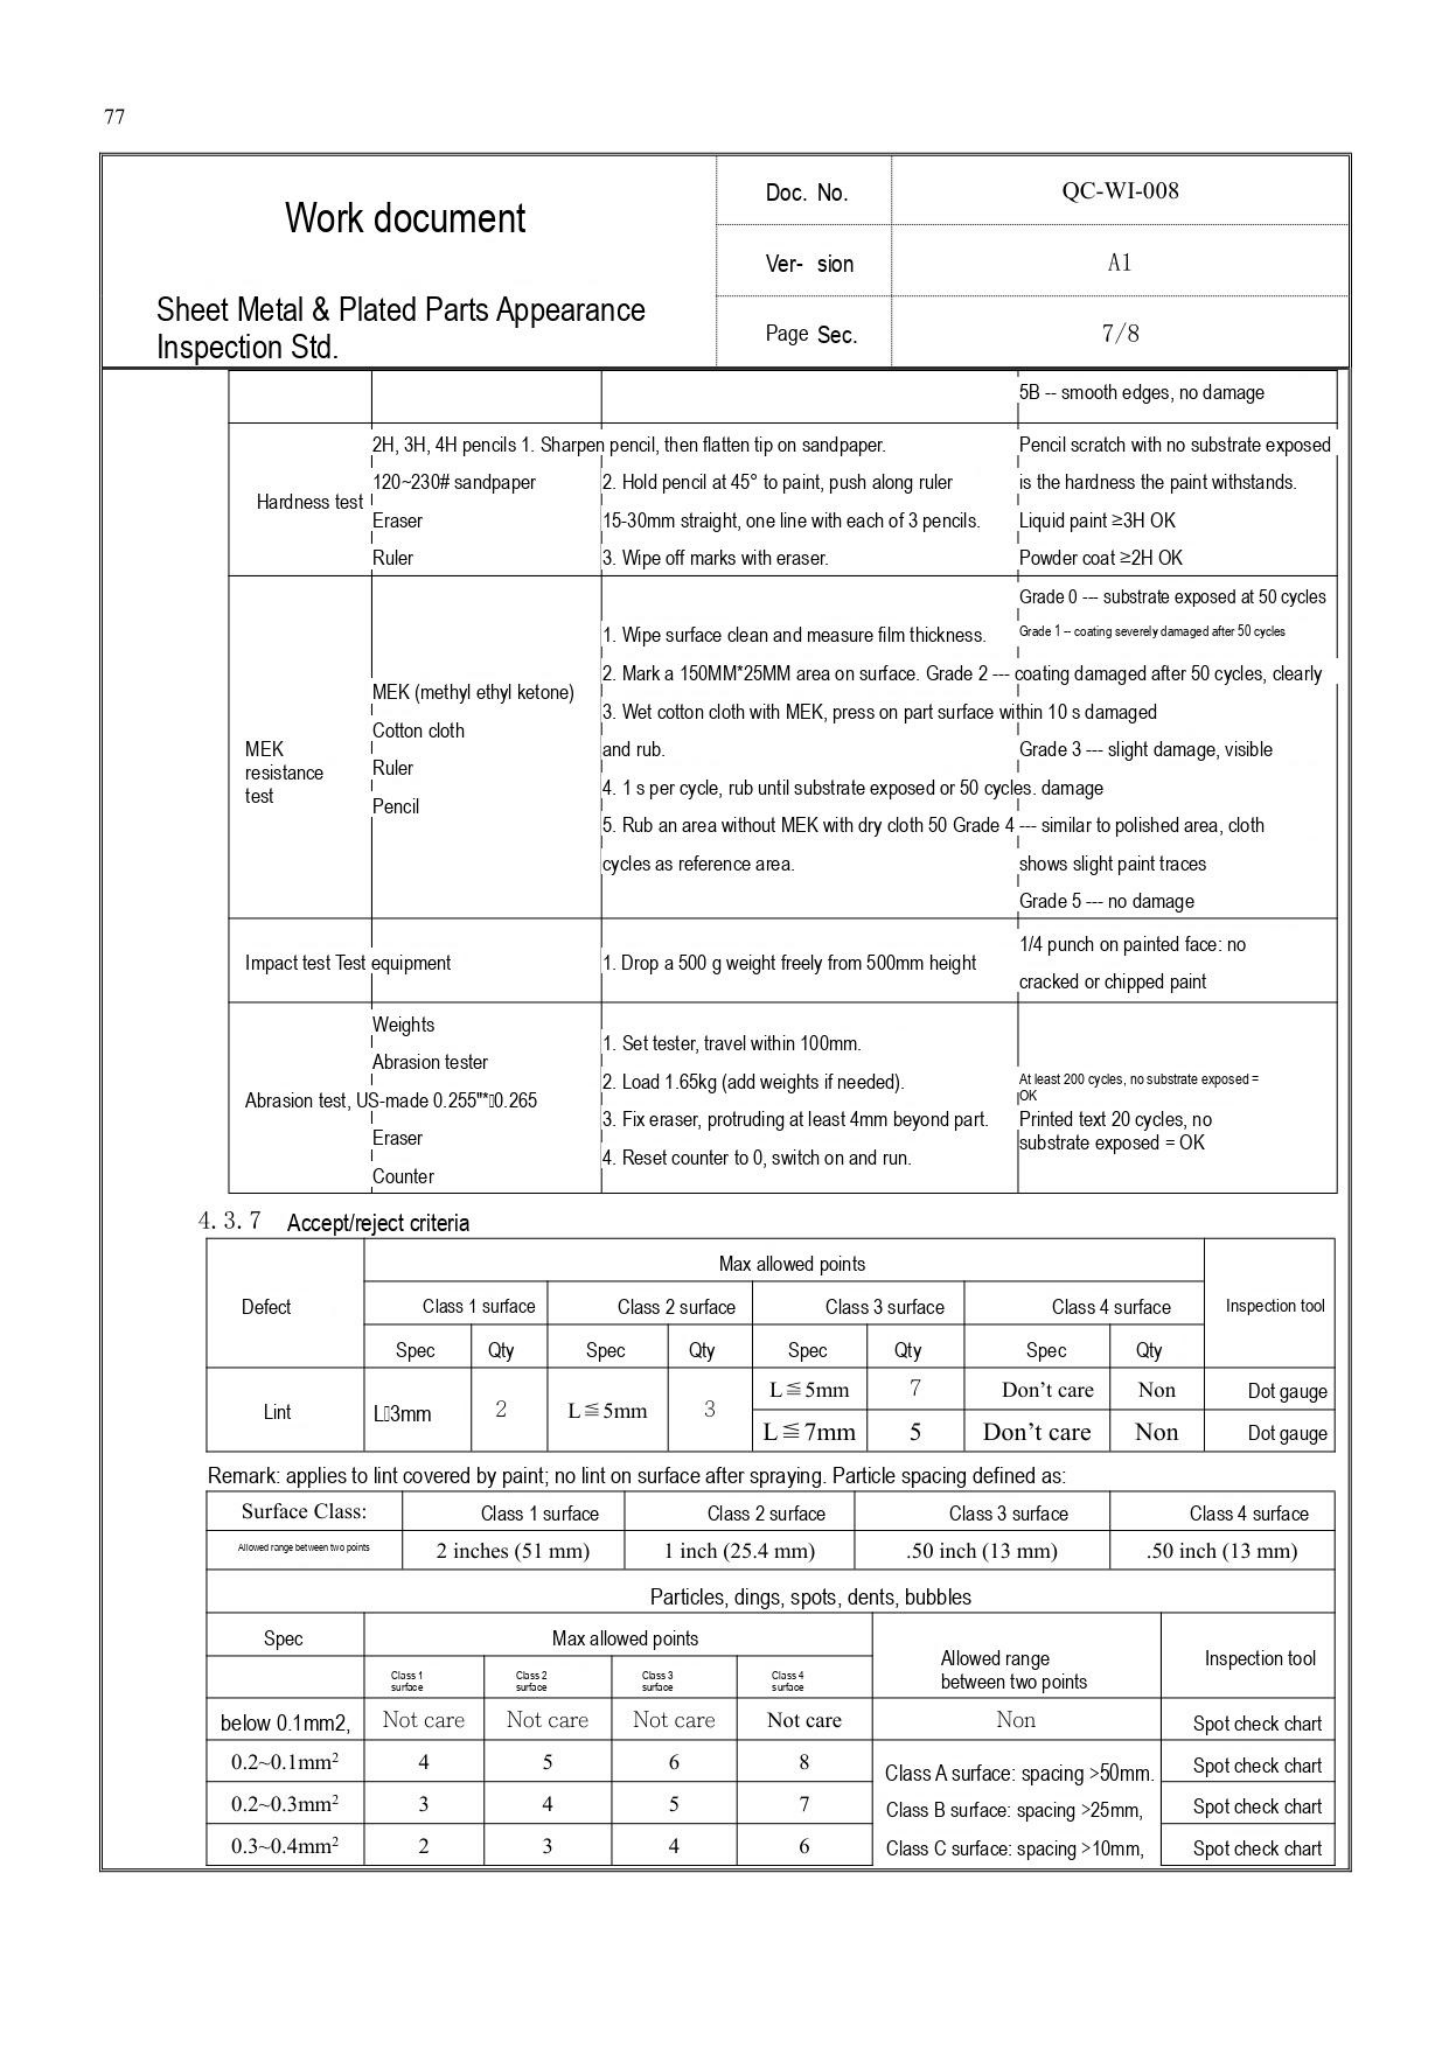77

| Work document<br>Sheet Metal & Plated Parts Appearance Inspection Std. | Doc. No. | QC-WI-008 |
|---|---|---|
| | Ver- sion | A1 |
| | Page Sec. | 7/8 |

| | | | |
|---|---|---|---|
| | | | 5B -- smooth edges, no damage |
| Hardness test | 2H, 3H, 4H pencils<br>120~230# sandpaper<br>Eraser<br>Ruler | 1. Sharpen pencil, then flatten tip on sandpaper.<br>2. Hold pencil at 45° to paint, push along ruler 15-30mm straight, one line with each of 3 pencils.<br>3. Wipe off marks with eraser. | Pencil scratch with no substrate exposed is the hardness the paint withstands.<br>Liquid paint ≥3H OK<br>Powder coat ≥2H OK |
| MEK resistance test | MEK (methyl ethyl ketone)<br>Cotton cloth<br>Ruler<br>Pencil | 1. Wipe surface clean and measure film thickness.<br>2. Mark a 150MM*25MM area on surface.<br>3. Wet cotton cloth with MEK, press on part surface within 10 s and rub.<br>4. 1 s per cycle, rub until substrate exposed or 50 cycles.<br>5. Rub an area without MEK with dry cloth 50 cycles as reference area. | Grade 0 --- substrate exposed at 50 cycles<br>Grade 1 -- coating severely damaged after 50 cycles<br>Grade 2 --- coating damaged after 50 cycles, clearly damaged<br>Grade 3 --- slight damage, visible damage<br>Grade 4 --- similar to polished area, cloth shows slight paint traces<br>Grade 5 --- no damage |
| Impact test | Test equipment | 1. Drop a 500 g weight freely from 500mm height | 1/4 punch on painted face: no cracked or chipped paint |
| Abrasion test, | Weights<br>Abrasion tester<br>US-made 0.255"*0.265<br>Eraser<br>Counter | 1. Set tester, travel within 100mm.<br>2. Load 1.65kg (add weights if needed).<br>3. Fix eraser, protruding at least 4mm beyond part.<br>4. Reset counter to 0, switch on and run. | At least 200 cycles, no substrate exposed = OK<br>Printed text 20 cycles, no substrate exposed = OK |

4.3.7 Accept/reject criteria

| Defect | Max allowed points | | | | | | | | Inspection tool |
|---|---|---|---|---|---|---|---|---|---|
| | Class 1 surface | | Class 2 surface | | Class 3 surface | | Class 4 surface | | |
| | Spec | Qty | Spec | Qty | Spec | Qty | Spec | Qty | |
| Lint | L3mm | 2 | L≦5mm | 3 | L≦5mm | 7 | Don't care | Non | Dot gauge |
| | | | | | L≦7mm | 5 | Don't care | Non | Dot gauge |

Remark: applies to lint covered by paint; no lint on surface after spraying. Particle spacing defined as:

| Surface Class: | Class 1 surface | Class 2 surface | Class 3 surface | Class 4 surface |
|---|---|---|---|---|
| Allowed range between two points | 2 inches (51 mm) | 1 inch (25.4 mm) | .50 inch (13 mm) | .50 inch (13 mm) |

Particles, dings, spots, dents, bubbles

| Spec | Max allowed points | | | | Allowed range between two points | Inspection tool |
|---|---|---|---|---|---|---|
| | Class 1 surface | Class 2 surface | Class 3 surface | Class 4 surface | | |
| below 0.1mm2, | Not care | Not care | Not care | Not care | Non | Spot check chart |
| 0.2~0.1mm² | 4 | 5 | 6 | 8 | Class A surface: spacing >50mm. | Spot check chart |
| 0.2~0.3mm² | 3 | 4 | 5 | 7 | Class B surface: spacing >25mm, | Spot check chart |
| 0.3~0.4mm² | 2 | 3 | 4 | 6 | Class C surface: spacing >10mm, | Spot check chart |
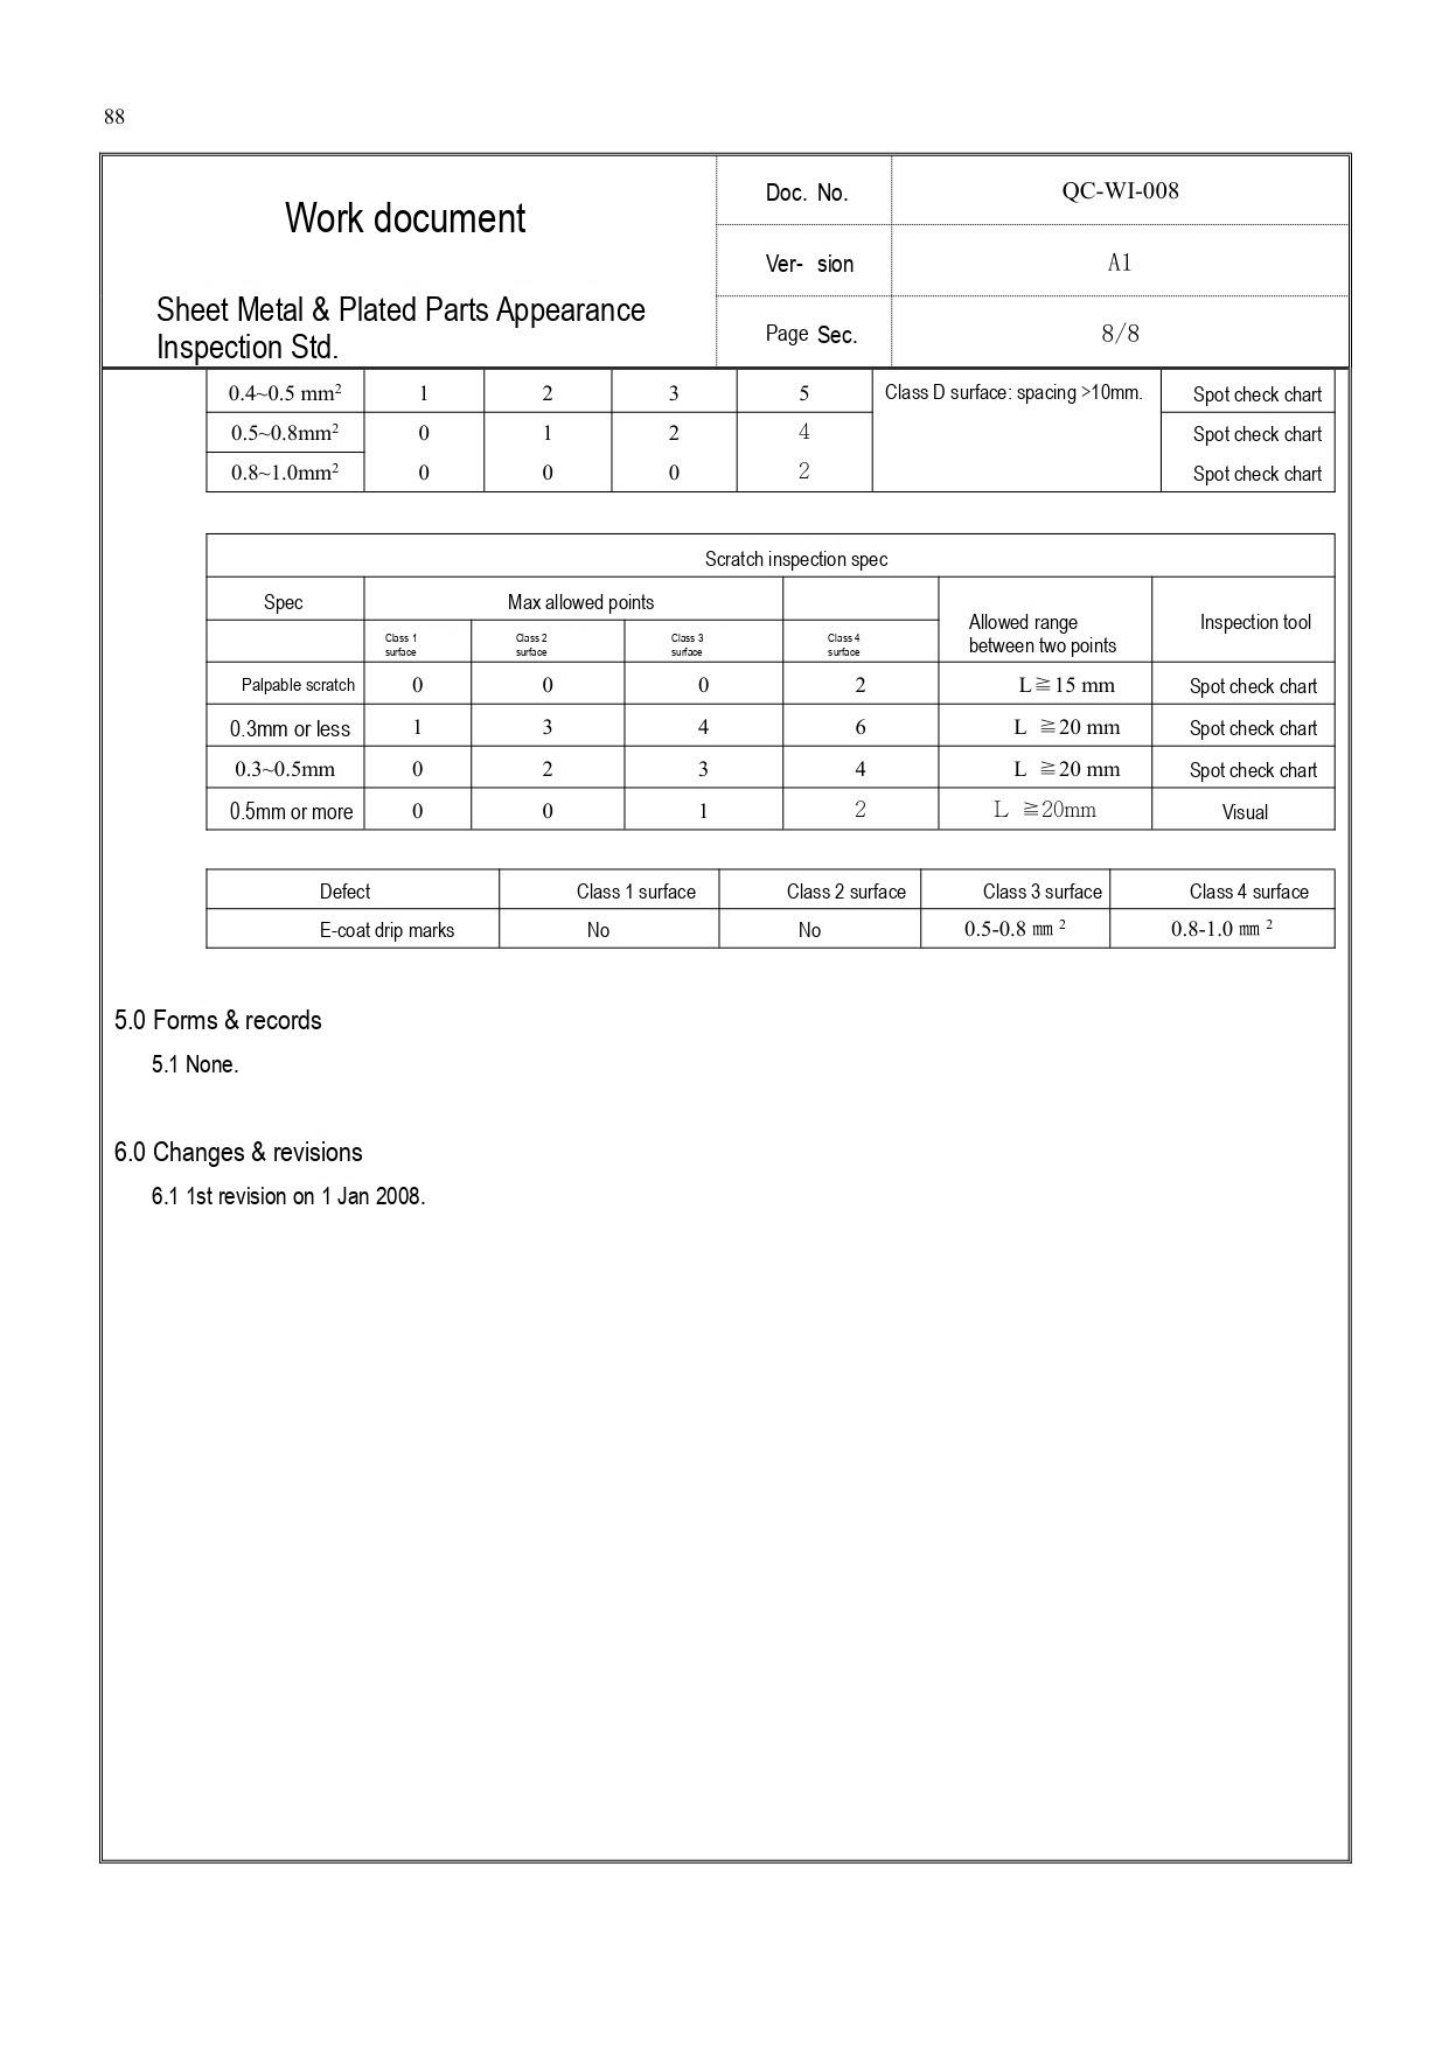88

| Work document<br><br>Sheet Metal & Plated Parts Appearance Inspection Std. | Doc. No. | QC-WI-008 |
|---|---|---|
| | Ver- sion | A1 |
| | Page Sec. | 8/8 |

| 0.4~0.5 mm² | 1 | 2 | 3 | 5 | Class D surface: spacing >10mm. | Spot check chart |
|---|---|---|---|---|---|---|
| 0.5~0.8mm² | 0 | 1 | 2 | 4 | | Spot check chart |
| 0.8~1.0mm² | 0 | 0 | 0 | 2 | | Spot check chart |

| Scratch inspection spec | | | | | | |
|---|---|---|---|---|---|---|
| Spec | Max allowed points | | | | Allowed range between two points | Inspection tool |
| | Class 1 surface | Class 2 surface | Class 3 surface | Class 4 surface | | |
| Palpable scratch | 0 | 0 | 0 | 2 | L≧15 mm | Spot check chart |
| 0.3mm or less | 1 | 3 | 4 | 6 | L ≧20 mm | Spot check chart |
| 0.3~0.5mm | 0 | 2 | 3 | 4 | L ≧20 mm | Spot check chart |
| 0.5mm or more | 0 | 0 | 1 | 2 | L ≧20mm | Visual |

| Defect | Class 1 surface | Class 2 surface | Class 3 surface | Class 4 surface |
|---|---|---|---|---|
| E-coat drip marks | No | No | 0.5-0.8 ㎜ ² | 0.8-1.0 ㎜ ² |

5.0 Forms & records

5.1 None.

6.0 Changes & revisions

6.1 1st revision on 1 Jan 2008.